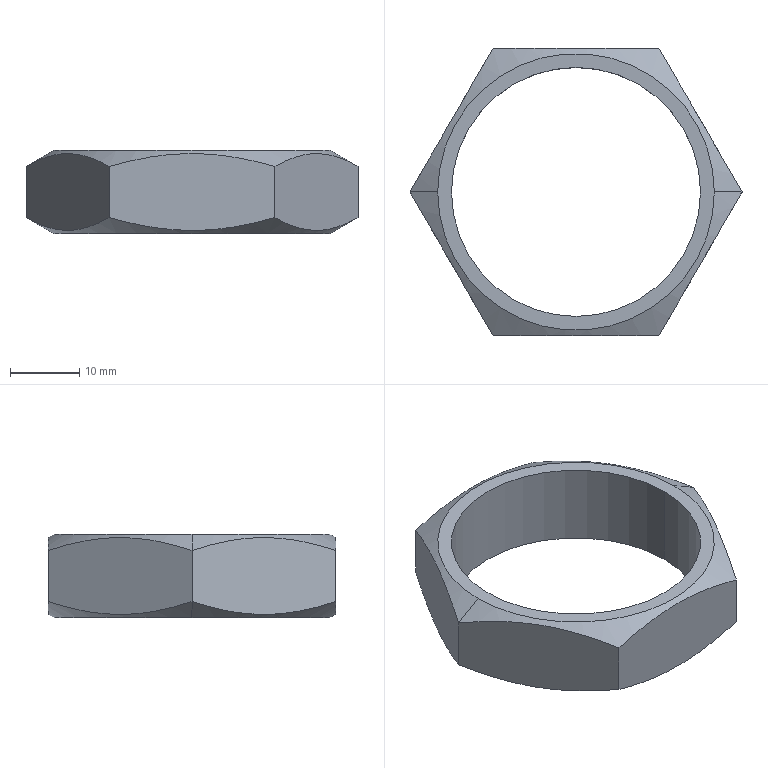Part | SolidWorks | features Extrusion 1, RevCut 1 | 1 solid | 14 faces | box 48 x 41.569 x 12 mm | volume 5415 mm3 | plane 8 | cone 4 | cylinder 2 | commonest cylinder face diameters 36 x2
STEP:
#1=CARTESIAN_POINT('',(-20.,0.,12.));
#2=VERTEX_POINT('',#1);
#3=CARTESIAN_POINT('',(20.,0.,12.));
#4=VERTEX_POINT('',#3);
#5=CARTESIAN_POINT('',(0.,0.,12.));
#6=DIRECTION('',(0.,0.,-1.));
#7=DIRECTION('',(-1.,0.,0.));
#8=AXIS2_PLACEMENT_3D('',#5,#6,#7);
#9=CIRCLE('',#8,20.);
#10=EDGE_CURVE('',#2,#4,#9,.T.);
#11=ORIENTED_EDGE('',*,*,#10,.T.);
#12=CARTESIAN_POINT('',(24.,0.,9.691));
#13=VERTEX_POINT('',#12);
#14=CARTESIAN_POINT('',(20.,0.,12.));
#15=DIRECTION('',(0.866,0.,-0.5));
#16=VECTOR('',#15,1000.);
#17=LINE('',#14,#16);
#18=EDGE_CURVE('',#4,#13,#17,.T.);
#19=ORIENTED_EDGE('',*,*,#18,.T.);
#20=CARTESIAN_POINT('',(12.,20.785,9.691));
#21=VERTEX_POINT('',#20);
#22=CARTESIAN_POINT('',(12.,20.785,9.691));
#23=CARTESIAN_POINT('',(12.98,19.088,10.256));
#24=CARTESIAN_POINT('',(13.967,17.379,10.722));
#25=CARTESIAN_POINT('',(15.961,13.924,11.368));
#26=CARTESIAN_POINT('',(16.968,12.179,11.546));
#27=CARTESIAN_POINT('',(18.244,9.97,11.547));
#28=CARTESIAN_POINT('',(18.5,9.526,11.537));
#29=CARTESIAN_POINT('',(19.01,8.642,11.494));
#30=CARTESIAN_POINT('',(19.265,8.202,11.462));
#31=CARTESIAN_POINT('',(20.025,6.885,11.335));
#32=CARTESIAN_POINT('',(20.528,6.013,11.209));
#33=CARTESIAN_POINT('',(22.03,3.412,10.724));
#34=CARTESIAN_POINT('',(23.019,1.699,10.257));
#35=CARTESIAN_POINT('',(24.,0.,9.691));
#36=B_SPLINE_CURVE_WITH_KNOTS('',3,(#22,#23,#24,#25,#26,#27,#28,#29,#30,#31,#32,#33,#34,#35),.UNSPECIFIED.,.F.,.F.,(4,2,2,2,2,2,4),(0.000000238,0.00606,0.01212,0.01363,0.01515,0.01818,0.02424),.UNSPECIFIED.);
#37=EDGE_CURVE('',#21,#13,#36,.T.);
#38=ORIENTED_EDGE('',*,*,#37,.F.);
#39=CARTESIAN_POINT('',(-12.,20.785,9.691));
#40=VERTEX_POINT('',#39);
#41=CARTESIAN_POINT('',(-12.,20.785,9.691));
#42=CARTESIAN_POINT('',(-11.024,20.785,9.972));
#43=CARTESIAN_POINT('',(-10.039,20.785,10.231));
#44=CARTESIAN_POINT('',(-8.046,20.785,10.69));
#45=CARTESIAN_POINT('',(-7.046,20.785,10.888));
#46=CARTESIAN_POINT('',(-4.04,20.785,11.373));
#47=CARTESIAN_POINT('',(-2.025,20.785,11.547));
#48=CARTESIAN_POINT('',(1.018,20.785,11.547));
#49=CARTESIAN_POINT('',(2.035,20.785,11.504));
#50=CARTESIAN_POINT('',(4.076,20.785,11.332));
#51=CARTESIAN_POINT('',(5.089,20.785,11.205));
#52=CARTESIAN_POINT('',(8.095,20.785,10.717));
#53=CARTESIAN_POINT('',(10.06,20.785,10.251));
#54=CARTESIAN_POINT('',(12.,20.785,9.691));
#55=B_SPLINE_CURVE_WITH_KNOTS('',3,(#41,#42,#43,#44,#45,#46,#47,#48,#49,#50,#51,#52,#53,#54),.UNSPECIFIED.,.F.,.F.,(4,2,2,2,2,2,4),(0.02134,0.02438,0.02741,0.03348,0.03652,0.03955,0.04562),.UNSPECIFIED.);
#56=EDGE_CURVE('',#40,#21,#55,.T.);
#57=ORIENTED_EDGE('',*,*,#56,.F.);
#58=CARTESIAN_POINT('',(-24.,0.,9.691));
#59=VERTEX_POINT('',#58);
#60=CARTESIAN_POINT('',(-24.,0.,9.691));
#61=CARTESIAN_POINT('',(-23.02,1.697,10.256));
#62=CARTESIAN_POINT('',(-22.033,3.406,10.722));
#63=CARTESIAN_POINT('',(-20.039,6.86,11.368));
#64=CARTESIAN_POINT('',(-19.032,8.605,11.546));
#65=CARTESIAN_POINT('',(-17.756,10.814,11.547));
#66=CARTESIAN_POINT('',(-17.5,11.258,11.537));
#67=CARTESIAN_POINT('',(-16.99,12.142,11.494));
#68=CARTESIAN_POINT('',(-16.735,12.583,11.462));
#69=CARTESIAN_POINT('',(-15.975,13.9,11.335));
#70=CARTESIAN_POINT('',(-15.472,14.772,11.209));
#71=CARTESIAN_POINT('',(-13.97,17.372,10.724));
#72=CARTESIAN_POINT('',(-12.981,19.086,10.257));
#73=CARTESIAN_POINT('',(-12.,20.785,9.691));
#74=B_SPLINE_CURVE_WITH_KNOTS('',3,(#60,#61,#62,#63,#64,#65,#66,#67,#68,#69,#70,#71,#72,#73),.UNSPECIFIED.,.F.,.F.,(4,2,2,2,2,2,4),(0.000000238,0.00606,0.01212,0.01363,0.01515,0.01818,0.02424),.UNSPECIFIED.);
#75=EDGE_CURVE('',#59,#40,#74,.T.);
#76=ORIENTED_EDGE('',*,*,#75,.F.);
#77=CARTESIAN_POINT('',(-20.,0.,12.));
#78=DIRECTION('',(-0.866,0.,-0.5));
#79=VECTOR('',#78,1000.);
#80=LINE('',#77,#79);
#81=EDGE_CURVE('',#2,#59,#80,.T.);
#82=ORIENTED_EDGE('',*,*,#81,.F.);
#83=EDGE_LOOP('',(#11,#19,#38,#57,#76,#82));
#84=FACE_OUTER_BOUND('',#83,.T.);
#85=CARTESIAN_POINT('',(0.,0.,12.));
#86=DIRECTION('',(0.,0.,-1.));
#87=DIRECTION('',(-1.,0.,0.));
#88=AXIS2_PLACEMENT_3D('',#85,#86,#87);
#89=CONICAL_SURFACE('',#88,20.,1.047);
#90=ADVANCED_FACE('',(#84),#89,.T.);
#91=CARTESIAN_POINT('',(-20.,0.,0.));
#92=VERTEX_POINT('',#91);
#93=CARTESIAN_POINT('',(20.,0.,0.));
#94=VERTEX_POINT('',#93);
#95=CARTESIAN_POINT('',(0.,0.,0.));
#96=DIRECTION('',(0.,0.,-1.));
#97=DIRECTION('',(-1.,0.,0.));
#98=AXIS2_PLACEMENT_3D('',#95,#96,#97);
#99=CIRCLE('',#98,20.);
#100=EDGE_CURVE('',#92,#94,#99,.T.);
#101=ORIENTED_EDGE('',*,*,#100,.F.);
#102=CARTESIAN_POINT('',(-24.,0.,2.309));
#103=VERTEX_POINT('',#102);
#104=CARTESIAN_POINT('',(-24.,0.,2.309));
#105=DIRECTION('',(-0.866,0.,0.5));
#106=VECTOR('',#105,1000.);
#107=LINE('',#104,#106);
#108=EDGE_CURVE('',#92,#103,#107,.T.);
#109=ORIENTED_EDGE('',*,*,#108,.T.);
#110=CARTESIAN_POINT('',(-12.,20.785,2.309));
#111=VERTEX_POINT('',#110);
#112=CARTESIAN_POINT('',(-12.,20.785,2.309));
#113=CARTESIAN_POINT('',(-12.98,19.088,1.744));
#114=CARTESIAN_POINT('',(-13.967,17.379,1.278));
#115=CARTESIAN_POINT('',(-15.961,13.924,0.6318));
#116=CARTESIAN_POINT('',(-16.968,12.179,0.4543));
#117=CARTESIAN_POINT('',(-18.244,9.97,0.4527));
#118=CARTESIAN_POINT('',(-18.5,9.526,0.4633));
#119=CARTESIAN_POINT('',(-19.01,8.642,0.506));
#120=CARTESIAN_POINT('',(-19.265,8.202,0.538));
#121=CARTESIAN_POINT('',(-20.025,6.885,0.6649));
#122=CARTESIAN_POINT('',(-20.528,6.013,0.7906));
#123=CARTESIAN_POINT('',(-22.03,3.412,1.276));
#124=CARTESIAN_POINT('',(-23.019,1.699,1.743));
#125=CARTESIAN_POINT('',(-24.,0.,2.309));
#126=B_SPLINE_CURVE_WITH_KNOTS('',3,(#112,#113,#114,#115,#116,#117,#118,#119,#120,#121,#122,#123,#124,#125),.UNSPECIFIED.,.F.,.F.,(4,2,2,2,2,2,4),(0.000000238,0.00606,0.01212,0.01363,0.01515,0.01818,0.02424),.UNSPECIFIED.);
#127=EDGE_CURVE('',#111,#103,#126,.T.);
#128=ORIENTED_EDGE('',*,*,#127,.F.);
#129=CARTESIAN_POINT('',(12.,20.785,2.309));
#130=VERTEX_POINT('',#129);
#131=CARTESIAN_POINT('',(12.,20.785,2.309));
#132=CARTESIAN_POINT('',(10.06,20.785,1.749));
#133=CARTESIAN_POINT('',(8.095,20.785,1.283));
#134=CARTESIAN_POINT('',(5.089,20.785,0.795));
#135=CARTESIAN_POINT('',(4.076,20.785,0.6676));
#136=CARTESIAN_POINT('',(2.035,20.785,0.4963));
#137=CARTESIAN_POINT('',(1.018,20.785,0.4531));
#138=CARTESIAN_POINT('',(-2.025,20.785,0.4528));
#139=CARTESIAN_POINT('',(-4.04,20.785,0.627));
#140=CARTESIAN_POINT('',(-7.046,20.785,1.112));
#141=CARTESIAN_POINT('',(-8.046,20.785,1.31));
#142=CARTESIAN_POINT('',(-10.039,20.785,1.769));
#143=CARTESIAN_POINT('',(-11.024,20.785,2.028));
#144=CARTESIAN_POINT('',(-12.,20.785,2.309));
#145=B_SPLINE_CURVE_WITH_KNOTS('',3,(#131,#132,#133,#134,#135,#136,#137,#138,#139,#140,#141,#142,#143,#144),.UNSPECIFIED.,.F.,.F.,(4,2,2,2,2,2,4),(0.008871,0.01493,0.01796,0.02098,0.02704,0.03007,0.0331),.UNSPECIFIED.);
#146=EDGE_CURVE('',#130,#111,#145,.T.);
#147=ORIENTED_EDGE('',*,*,#146,.F.);
#148=CARTESIAN_POINT('',(24.,0.,2.309));
#149=VERTEX_POINT('',#148);
#150=CARTESIAN_POINT('',(24.,0.,2.309));
#151=CARTESIAN_POINT('',(23.02,1.697,1.744));
#152=CARTESIAN_POINT('',(22.033,3.406,1.278));
#153=CARTESIAN_POINT('',(20.039,6.86,0.6318));
#154=CARTESIAN_POINT('',(19.032,8.605,0.4543));
#155=CARTESIAN_POINT('',(17.756,10.814,0.4527));
#156=CARTESIAN_POINT('',(17.5,11.258,0.4633));
#157=CARTESIAN_POINT('',(16.99,12.142,0.506));
#158=CARTESIAN_POINT('',(16.735,12.583,0.538));
#159=CARTESIAN_POINT('',(15.975,13.9,0.6649));
#160=CARTESIAN_POINT('',(15.472,14.772,0.7906));
#161=CARTESIAN_POINT('',(13.97,17.372,1.276));
#162=CARTESIAN_POINT('',(12.981,19.086,1.743));
#163=CARTESIAN_POINT('',(12.,20.785,2.309));
#164=B_SPLINE_CURVE_WITH_KNOTS('',3,(#150,#151,#152,#153,#154,#155,#156,#157,#158,#159,#160,#161,#162,#163),.UNSPECIFIED.,.F.,.F.,(4,2,2,2,2,2,4),(0.000000238,0.00606,0.01212,0.01363,0.01515,0.01818,0.02424),.UNSPECIFIED.);
#165=EDGE_CURVE('',#149,#130,#164,.T.);
#166=ORIENTED_EDGE('',*,*,#165,.F.);
#167=CARTESIAN_POINT('',(24.,0.,2.309));
#168=DIRECTION('',(0.866,0.,0.5));
#169=VECTOR('',#168,1000.);
#170=LINE('',#167,#169);
#171=EDGE_CURVE('',#94,#149,#170,.T.);
#172=ORIENTED_EDGE('',*,*,#171,.F.);
#173=EDGE_LOOP('',(#101,#109,#128,#147,#166,#172));
#174=FACE_OUTER_BOUND('',#173,.T.);
#175=CARTESIAN_POINT('',(0.,0.,2.309));
#176=DIRECTION('',(0.,0.,1.));
#177=DIRECTION('',(1.,0.,0.));
#178=AXIS2_PLACEMENT_3D('',#175,#176,#177);
#179=CONICAL_SURFACE('',#178,24.,1.047);
#180=ADVANCED_FACE('',(#174),#179,.T.);
#181=CARTESIAN_POINT('',(-18.,0.,12.));
#182=VERTEX_POINT('',#181);
#183=CARTESIAN_POINT('',(18.,0.,12.));
#184=VERTEX_POINT('',#183);
#185=CARTESIAN_POINT('',(0.,0.,12.));
#186=DIRECTION('',(0.,0.,1.));
#187=DIRECTION('',(1.,0.,0.));
#188=AXIS2_PLACEMENT_3D('',#185,#186,#187);
#189=CIRCLE('',#188,18.);
#190=EDGE_CURVE('',#182,#184,#189,.T.);
#191=ORIENTED_EDGE('',*,*,#190,.T.);
#192=CARTESIAN_POINT('',(18.,0.,0.));
#193=VERTEX_POINT('',#192);
#194=CARTESIAN_POINT('',(18.,0.,12.));
#195=DIRECTION('',(0.,0.,-1.));
#196=VECTOR('',#195,1000.);
#197=LINE('',#194,#196);
#198=EDGE_CURVE('',#184,#193,#197,.T.);
#199=ORIENTED_EDGE('',*,*,#198,.T.);
#200=CARTESIAN_POINT('',(-18.,0.,0.));
#201=VERTEX_POINT('',#200);
#202=CARTESIAN_POINT('',(0.,0.,0.));
#203=DIRECTION('',(0.,0.,1.));
#204=DIRECTION('',(1.,0.,0.));
#205=AXIS2_PLACEMENT_3D('',#202,#203,#204);
#206=CIRCLE('',#205,18.);
#207=EDGE_CURVE('',#201,#193,#206,.T.);
#208=ORIENTED_EDGE('',*,*,#207,.F.);
#209=CARTESIAN_POINT('',(-18.,0.,12.));
#210=DIRECTION('',(0.,0.,-1.));
#211=VECTOR('',#210,1000.);
#212=LINE('',#209,#211);
#213=EDGE_CURVE('',#182,#201,#212,.T.);
#214=ORIENTED_EDGE('',*,*,#213,.F.);
#215=EDGE_LOOP('',(#191,#199,#208,#214));
#216=FACE_OUTER_BOUND('',#215,.T.);
#217=CARTESIAN_POINT('',(0.,0.,12.));
#218=DIRECTION('',(0.,0.,-1.));
#219=DIRECTION('',(-1.,0.,0.));
#220=AXIS2_PLACEMENT_3D('',#217,#218,#219);
#221=CYLINDRICAL_SURFACE('',#220,18.);
#222=ADVANCED_FACE('',(#216),#221,.F.);
#223=ORIENTED_EDGE('',*,*,#207,.T.);
#224=CARTESIAN_POINT('',(0.,0.,0.));
#225=DIRECTION('',(0.,0.,1.));
#226=DIRECTION('',(1.,0.,0.));
#227=AXIS2_PLACEMENT_3D('',#224,#225,#226);
#228=CIRCLE('',#227,18.);
#229=EDGE_CURVE('',#193,#201,#228,.T.);
#230=ORIENTED_EDGE('',*,*,#229,.T.);
#231=EDGE_LOOP('',(#223,#230));
#232=FACE_BOUND('',#231,.T.);
#233=CARTESIAN_POINT('',(0.,0.,0.));
#234=DIRECTION('',(0.,0.,-1.));
#235=DIRECTION('',(-1.,0.,0.));
#236=AXIS2_PLACEMENT_3D('',#233,#234,#235);
#237=CIRCLE('',#236,20.);
#238=EDGE_CURVE('',#94,#92,#237,.T.);
#239=ORIENTED_EDGE('',*,*,#238,.T.);
#240=ORIENTED_EDGE('',*,*,#100,.T.);
#241=EDGE_LOOP('',(#239,#240));
#242=FACE_OUTER_BOUND('',#241,.T.);
#243=CARTESIAN_POINT('',(0.,0.,0.));
#244=DIRECTION('',(0.,0.,1.));
#245=DIRECTION('',(1.,0.,0.));
#246=AXIS2_PLACEMENT_3D('',#243,#244,#245);
#247=PLANE('',#246);
#248=ADVANCED_FACE('',(#232,#242),#247,.F.);
#249=ORIENTED_EDGE('',*,*,#10,.F.);
#250=CARTESIAN_POINT('',(0.,0.,12.));
#251=DIRECTION('',(0.,0.,-1.));
#252=DIRECTION('',(-1.,0.,0.));
#253=AXIS2_PLACEMENT_3D('',#250,#251,#252);
#254=CIRCLE('',#253,20.);
#255=EDGE_CURVE('',#4,#2,#254,.T.);
#256=ORIENTED_EDGE('',*,*,#255,.F.);
#257=EDGE_LOOP('',(#249,#256));
#258=FACE_OUTER_BOUND('',#257,.T.);
#259=ORIENTED_EDGE('',*,*,#190,.F.);
#260=CARTESIAN_POINT('',(0.,0.,12.));
#261=DIRECTION('',(0.,0.,1.));
#262=DIRECTION('',(1.,0.,0.));
#263=AXIS2_PLACEMENT_3D('',#260,#261,#262);
#264=CIRCLE('',#263,18.);
#265=EDGE_CURVE('',#184,#182,#264,.T.);
#266=ORIENTED_EDGE('',*,*,#265,.F.);
#267=EDGE_LOOP('',(#259,#266));
#268=FACE_BOUND('',#267,.T.);
#269=CARTESIAN_POINT('',(0.,0.,12.));
#270=DIRECTION('',(0.,0.,1.));
#271=DIRECTION('',(1.,0.,0.));
#272=AXIS2_PLACEMENT_3D('',#269,#270,#271);
#273=PLANE('',#272);
#274=ADVANCED_FACE('',(#258,#268),#273,.T.);
#275=CARTESIAN_POINT('',(24.,0.,12.));
#276=DIRECTION('',(0.,0.,-1.));
#277=VECTOR('',#276,1000.);
#278=LINE('',#275,#277);
#279=EDGE_CURVE('',#13,#149,#278,.T.);
#280=ORIENTED_EDGE('',*,*,#279,.F.);
#281=CARTESIAN_POINT('',(12.,-20.785,9.691));
#282=VERTEX_POINT('',#281);
#283=CARTESIAN_POINT('',(24.,0.,9.691));
#284=CARTESIAN_POINT('',(23.02,-1.697,10.256));
#285=CARTESIAN_POINT('',(22.033,-3.406,10.722));
#286=CARTESIAN_POINT('',(20.039,-6.86,11.368));
#287=CARTESIAN_POINT('',(19.032,-8.605,11.546));
#288=CARTESIAN_POINT('',(17.756,-10.814,11.547));
#289=CARTESIAN_POINT('',(17.5,-11.258,11.537));
#290=CARTESIAN_POINT('',(16.99,-12.142,11.494));
#291=CARTESIAN_POINT('',(16.735,-12.583,11.462));
#292=CARTESIAN_POINT('',(15.975,-13.9,11.335));
#293=CARTESIAN_POINT('',(15.472,-14.772,11.209));
#294=CARTESIAN_POINT('',(13.97,-17.372,10.724));
#295=CARTESIAN_POINT('',(12.981,-19.086,10.257));
#296=CARTESIAN_POINT('',(12.,-20.785,9.691));
#297=B_SPLINE_CURVE_WITH_KNOTS('',3,(#283,#284,#285,#286,#287,#288,#289,#290,#291,#292,#293,#294,#295,#296),.UNSPECIFIED.,.F.,.F.,(4,2,2,2,2,2,4),(0.000000238,0.00606,0.01212,0.01363,0.01515,0.01818,0.02424),.UNSPECIFIED.);
#298=EDGE_CURVE('',#13,#282,#297,.T.);
#299=ORIENTED_EDGE('',*,*,#298,.T.);
#300=CARTESIAN_POINT('',(12.,-20.785,2.309));
#301=VERTEX_POINT('',#300);
#302=CARTESIAN_POINT('',(12.,-20.785,12.));
#303=DIRECTION('',(0.,0.,-1.));
#304=VECTOR('',#303,1000.);
#305=LINE('',#302,#304);
#306=EDGE_CURVE('',#282,#301,#305,.T.);
#307=ORIENTED_EDGE('',*,*,#306,.T.);
#308=CARTESIAN_POINT('',(12.,-20.785,2.309));
#309=CARTESIAN_POINT('',(12.98,-19.088,1.744));
#310=CARTESIAN_POINT('',(13.967,-17.379,1.278));
#311=CARTESIAN_POINT('',(15.961,-13.924,0.6318));
#312=CARTESIAN_POINT('',(16.968,-12.179,0.4543));
#313=CARTESIAN_POINT('',(18.244,-9.97,0.4527));
#314=CARTESIAN_POINT('',(18.5,-9.526,0.4633));
#315=CARTESIAN_POINT('',(19.01,-8.642,0.506));
#316=CARTESIAN_POINT('',(19.265,-8.202,0.538));
#317=CARTESIAN_POINT('',(20.025,-6.885,0.6649));
#318=CARTESIAN_POINT('',(20.528,-6.013,0.7906));
#319=CARTESIAN_POINT('',(22.03,-3.412,1.276));
#320=CARTESIAN_POINT('',(23.019,-1.699,1.743));
#321=CARTESIAN_POINT('',(24.,0.,2.309));
#322=B_SPLINE_CURVE_WITH_KNOTS('',3,(#308,#309,#310,#311,#312,#313,#314,#315,#316,#317,#318,#319,#320,#321),.UNSPECIFIED.,.F.,.F.,(4,2,2,2,2,2,4),(0.000000238,0.00606,0.01212,0.01363,0.01515,0.01818,0.02424),.UNSPECIFIED.);
#323=EDGE_CURVE('',#301,#149,#322,.T.);
#324=ORIENTED_EDGE('',*,*,#323,.T.);
#325=EDGE_LOOP('',(#280,#299,#307,#324));
#326=FACE_OUTER_BOUND('',#325,.T.);
#327=CARTESIAN_POINT('',(12.,-20.785,12.));
#328=DIRECTION('',(-0.866,0.5,0.));
#329=DIRECTION('',(-0.5,-0.866,0.));
#330=AXIS2_PLACEMENT_3D('',#327,#328,#329);
#331=PLANE('',#330);
#332=ADVANCED_FACE('',(#326),#331,.F.);
#333=CARTESIAN_POINT('',(12.,20.785,12.));
#334=DIRECTION('',(0.,0.,-1.));
#335=VECTOR('',#334,1000.);
#336=LINE('',#333,#335);
#337=EDGE_CURVE('',#21,#130,#336,.T.);
#338=ORIENTED_EDGE('',*,*,#337,.F.);
#339=ORIENTED_EDGE('',*,*,#37,.T.);
#340=ORIENTED_EDGE('',*,*,#279,.T.);
#341=ORIENTED_EDGE('',*,*,#165,.T.);
#342=EDGE_LOOP('',(#338,#339,#340,#341));
#343=FACE_OUTER_BOUND('',#342,.T.);
#344=CARTESIAN_POINT('',(24.,0.,12.));
#345=DIRECTION('',(-0.866,-0.5,0.));
#346=DIRECTION('',(0.5,-0.866,0.));
#347=AXIS2_PLACEMENT_3D('',#344,#345,#346);
#348=PLANE('',#347);
#349=ADVANCED_FACE('',(#343),#348,.F.);
#350=CARTESIAN_POINT('',(-12.,20.785,12.));
#351=DIRECTION('',(0.,0.,-1.));
#352=VECTOR('',#351,1000.);
#353=LINE('',#350,#352);
#354=EDGE_CURVE('',#40,#111,#353,.T.);
#355=ORIENTED_EDGE('',*,*,#354,.F.);
#356=ORIENTED_EDGE('',*,*,#56,.T.);
#357=ORIENTED_EDGE('',*,*,#337,.T.);
#358=ORIENTED_EDGE('',*,*,#146,.T.);
#359=EDGE_LOOP('',(#355,#356,#357,#358));
#360=FACE_OUTER_BOUND('',#359,.T.);
#361=CARTESIAN_POINT('',(12.,20.785,12.));
#362=DIRECTION('',(0.,-1.,0.));
#363=DIRECTION('',(0.,0.,-1.));
#364=AXIS2_PLACEMENT_3D('',#361,#362,#363);
#365=PLANE('',#364);
#366=ADVANCED_FACE('',(#360),#365,.F.);
#367=CARTESIAN_POINT('',(-24.,0.,12.));
#368=DIRECTION('',(0.,0.,-1.));
#369=VECTOR('',#368,1000.);
#370=LINE('',#367,#369);
#371=EDGE_CURVE('',#59,#103,#370,.T.);
#372=ORIENTED_EDGE('',*,*,#371,.F.);
#373=ORIENTED_EDGE('',*,*,#75,.T.);
#374=ORIENTED_EDGE('',*,*,#354,.T.);
#375=ORIENTED_EDGE('',*,*,#127,.T.);
#376=EDGE_LOOP('',(#372,#373,#374,#375));
#377=FACE_OUTER_BOUND('',#376,.T.);
#378=CARTESIAN_POINT('',(-12.,20.785,12.));
#379=DIRECTION('',(0.866,-0.5,0.));
#380=DIRECTION('',(0.5,0.866,0.));
#381=AXIS2_PLACEMENT_3D('',#378,#379,#380);
#382=PLANE('',#381);
#383=ADVANCED_FACE('',(#377),#382,.F.);
#384=CARTESIAN_POINT('',(-12.,-20.785,9.691));
#385=VERTEX_POINT('',#384);
#386=CARTESIAN_POINT('',(-12.,-20.785,2.309));
#387=VERTEX_POINT('',#386);
#388=CARTESIAN_POINT('',(-12.,-20.785,12.));
#389=DIRECTION('',(0.,0.,-1.));
#390=VECTOR('',#389,1000.);
#391=LINE('',#388,#390);
#392=EDGE_CURVE('',#385,#387,#391,.T.);
#393=ORIENTED_EDGE('',*,*,#392,.F.);
#394=CARTESIAN_POINT('',(-12.,-20.785,9.691));
#395=CARTESIAN_POINT('',(-12.98,-19.088,10.256));
#396=CARTESIAN_POINT('',(-13.967,-17.379,10.722));
#397=CARTESIAN_POINT('',(-15.961,-13.924,11.368));
#398=CARTESIAN_POINT('',(-16.968,-12.179,11.546));
#399=CARTESIAN_POINT('',(-18.244,-9.97,11.547));
#400=CARTESIAN_POINT('',(-18.5,-9.526,11.537));
#401=CARTESIAN_POINT('',(-19.01,-8.642,11.494));
#402=CARTESIAN_POINT('',(-19.265,-8.202,11.462));
#403=CARTESIAN_POINT('',(-20.025,-6.885,11.335));
#404=CARTESIAN_POINT('',(-20.528,-6.013,11.209));
#405=CARTESIAN_POINT('',(-22.03,-3.412,10.724));
#406=CARTESIAN_POINT('',(-23.019,-1.699,10.257));
#407=CARTESIAN_POINT('',(-24.,0.,9.691));
#408=B_SPLINE_CURVE_WITH_KNOTS('',3,(#394,#395,#396,#397,#398,#399,#400,#401,#402,#403,#404,#405,#406,#407),.UNSPECIFIED.,.F.,.F.,(4,2,2,2,2,2,4),(0.000000238,0.00606,0.01212,0.01363,0.01515,0.01818,0.02424),.UNSPECIFIED.);
#409=EDGE_CURVE('',#385,#59,#408,.T.);
#410=ORIENTED_EDGE('',*,*,#409,.T.);
#411=ORIENTED_EDGE('',*,*,#371,.T.);
#412=CARTESIAN_POINT('',(-24.,0.,2.309));
#413=CARTESIAN_POINT('',(-23.02,-1.697,1.744));
#414=CARTESIAN_POINT('',(-22.033,-3.406,1.278));
#415=CARTESIAN_POINT('',(-20.039,-6.86,0.6318));
#416=CARTESIAN_POINT('',(-19.032,-8.605,0.4543));
#417=CARTESIAN_POINT('',(-17.756,-10.814,0.4527));
#418=CARTESIAN_POINT('',(-17.5,-11.258,0.4633));
#419=CARTESIAN_POINT('',(-16.99,-12.142,0.506));
#420=CARTESIAN_POINT('',(-16.735,-12.583,0.538));
#421=CARTESIAN_POINT('',(-15.975,-13.9,0.6649));
#422=CARTESIAN_POINT('',(-15.472,-14.772,0.7906));
#423=CARTESIAN_POINT('',(-13.97,-17.372,1.276));
#424=CARTESIAN_POINT('',(-12.981,-19.086,1.743));
#425=CARTESIAN_POINT('',(-12.,-20.785,2.309));
#426=B_SPLINE_CURVE_WITH_KNOTS('',3,(#412,#413,#414,#415,#416,#417,#418,#419,#420,#421,#422,#423,#424,#425),.UNSPECIFIED.,.F.,.F.,(4,2,2,2,2,2,4),(0.000000238,0.00606,0.01212,0.01363,0.01515,0.01818,0.02424),.UNSPECIFIED.);
#427=EDGE_CURVE('',#103,#387,#426,.T.);
#428=ORIENTED_EDGE('',*,*,#427,.T.);
#429=EDGE_LOOP('',(#393,#410,#411,#428));
#430=FACE_OUTER_BOUND('',#429,.T.);
#431=CARTESIAN_POINT('',(-24.,0.,12.));
#432=DIRECTION('',(0.866,0.5,0.));
#433=DIRECTION('',(-0.5,0.866,0.));
#434=AXIS2_PLACEMENT_3D('',#431,#432,#433);
#435=PLANE('',#434);
#436=ADVANCED_FACE('',(#430),#435,.F.);
#437=ORIENTED_EDGE('',*,*,#306,.F.);
#438=CARTESIAN_POINT('',(12.,-20.785,9.691));
#439=CARTESIAN_POINT('',(10.06,-20.785,10.251));
#440=CARTESIAN_POINT('',(8.095,-20.785,10.717));
#441=CARTESIAN_POINT('',(5.089,-20.785,11.205));
#442=CARTESIAN_POINT('',(4.076,-20.785,11.332));
#443=CARTESIAN_POINT('',(2.035,-20.785,11.504));
#444=CARTESIAN_POINT('',(1.018,-20.785,11.547));
#445=CARTESIAN_POINT('',(-2.025,-20.785,11.547));
#446=CARTESIAN_POINT('',(-4.04,-20.785,11.373));
#447=CARTESIAN_POINT('',(-7.046,-20.785,10.888));
#448=CARTESIAN_POINT('',(-8.046,-20.785,10.69));
#449=CARTESIAN_POINT('',(-10.039,-20.785,10.231));
#450=CARTESIAN_POINT('',(-11.024,-20.785,9.972));
#451=CARTESIAN_POINT('',(-12.,-20.785,9.691));
#452=B_SPLINE_CURVE_WITH_KNOTS('',3,(#438,#439,#440,#441,#442,#443,#444,#445,#446,#447,#448,#449,#450,#451),.UNSPECIFIED.,.F.,.F.,(4,2,2,2,2,2,4),(0.008871,0.01493,0.01796,0.02098,0.02704,0.03007,0.0331),.UNSPECIFIED.);
#453=EDGE_CURVE('',#282,#385,#452,.T.);
#454=ORIENTED_EDGE('',*,*,#453,.T.);
#455=ORIENTED_EDGE('',*,*,#392,.T.);
#456=CARTESIAN_POINT('',(-12.,-20.785,2.309));
#457=CARTESIAN_POINT('',(-11.024,-20.785,2.028));
#458=CARTESIAN_POINT('',(-10.039,-20.785,1.769));
#459=CARTESIAN_POINT('',(-8.046,-20.785,1.31));
#460=CARTESIAN_POINT('',(-7.046,-20.785,1.112));
#461=CARTESIAN_POINT('',(-4.04,-20.785,0.627));
#462=CARTESIAN_POINT('',(-2.025,-20.785,0.4528));
#463=CARTESIAN_POINT('',(1.018,-20.785,0.4531));
#464=CARTESIAN_POINT('',(2.035,-20.785,0.4963));
#465=CARTESIAN_POINT('',(4.076,-20.785,0.6676));
#466=CARTESIAN_POINT('',(5.089,-20.785,0.795));
#467=CARTESIAN_POINT('',(8.095,-20.785,1.283));
#468=CARTESIAN_POINT('',(10.06,-20.785,1.749));
#469=CARTESIAN_POINT('',(12.,-20.785,2.309));
#470=B_SPLINE_CURVE_WITH_KNOTS('',3,(#456,#457,#458,#459,#460,#461,#462,#463,#464,#465,#466,#467,#468,#469),.UNSPECIFIED.,.F.,.F.,(4,2,2,2,2,2,4),(0.02134,0.02438,0.02741,0.03348,0.03652,0.03955,0.04562),.UNSPECIFIED.);
#471=EDGE_CURVE('',#387,#301,#470,.T.);
#472=ORIENTED_EDGE('',*,*,#471,.T.);
#473=EDGE_LOOP('',(#437,#454,#455,#472));
#474=FACE_OUTER_BOUND('',#473,.T.);
#475=CARTESIAN_POINT('',(-12.,-20.785,12.));
#476=DIRECTION('',(0.,1.,0.));
#477=DIRECTION('',(0.,0.,1.));
#478=AXIS2_PLACEMENT_3D('',#475,#476,#477);
#479=PLANE('',#478);
#480=ADVANCED_FACE('',(#474),#479,.F.);
#481=ORIENTED_EDGE('',*,*,#198,.F.);
#482=ORIENTED_EDGE('',*,*,#265,.T.);
#483=ORIENTED_EDGE('',*,*,#213,.T.);
#484=ORIENTED_EDGE('',*,*,#229,.F.);
#485=EDGE_LOOP('',(#481,#482,#483,#484));
#486=FACE_OUTER_BOUND('',#485,.T.);
#487=CARTESIAN_POINT('',(0.,0.,12.));
#488=DIRECTION('',(0.,0.,-1.));
#489=DIRECTION('',(-1.,0.,0.));
#490=AXIS2_PLACEMENT_3D('',#487,#488,#489);
#491=CYLINDRICAL_SURFACE('',#490,18.);
#492=ADVANCED_FACE('',(#486),#491,.F.);
#493=ORIENTED_EDGE('',*,*,#108,.F.);
#494=ORIENTED_EDGE('',*,*,#238,.F.);
#495=ORIENTED_EDGE('',*,*,#171,.T.);
#496=ORIENTED_EDGE('',*,*,#323,.F.);
#497=ORIENTED_EDGE('',*,*,#471,.F.);
#498=ORIENTED_EDGE('',*,*,#427,.F.);
#499=EDGE_LOOP('',(#493,#494,#495,#496,#497,#498));
#500=FACE_OUTER_BOUND('',#499,.T.);
#501=CARTESIAN_POINT('',(0.,0.,2.309));
#502=DIRECTION('',(0.,0.,1.));
#503=DIRECTION('',(1.,0.,0.));
#504=AXIS2_PLACEMENT_3D('',#501,#502,#503);
#505=CONICAL_SURFACE('',#504,24.,1.047);
#506=ADVANCED_FACE('',(#500),#505,.T.);
#507=ORIENTED_EDGE('',*,*,#18,.F.);
#508=ORIENTED_EDGE('',*,*,#255,.T.);
#509=ORIENTED_EDGE('',*,*,#81,.T.);
#510=ORIENTED_EDGE('',*,*,#409,.F.);
#511=ORIENTED_EDGE('',*,*,#453,.F.);
#512=ORIENTED_EDGE('',*,*,#298,.F.);
#513=EDGE_LOOP('',(#507,#508,#509,#510,#511,#512));
#514=FACE_OUTER_BOUND('',#513,.T.);
#515=CARTESIAN_POINT('',(0.,0.,12.));
#516=DIRECTION('',(0.,0.,-1.));
#517=DIRECTION('',(-1.,0.,0.));
#518=AXIS2_PLACEMENT_3D('',#515,#516,#517);
#519=CONICAL_SURFACE('',#518,20.,1.047);
#520=ADVANCED_FACE('',(#514),#519,.T.);
#521=CLOSED_SHELL('',(#90,#180,#222,#248,#274,#332,#349,#366,#383,#436,#480,#492,#506,#520));
#522=MANIFOLD_SOLID_BREP('',#521);
#523=CARTESIAN_POINT('',(0.,0.,0.));
#524=DIRECTION('',(0.,0.,1.));
#525=DIRECTION('',(1.,0.,0.));
#526=AXIS2_PLACEMENT_3D('',#523,#524,#525);
#527=(LENGTH_UNIT()NAMED_UNIT(*)SI_UNIT(.MILLI.,.METRE.));
#528=UNCERTAINTY_MEASURE_WITH_UNIT(LENGTH_MEASURE(0.00001),#527,'','');
#529=(NAMED_UNIT(*)PLANE_ANGLE_UNIT()SI_UNIT($,.RADIAN.));
#530=(NAMED_UNIT(*)SI_UNIT($,.STERADIAN.)SOLID_ANGLE_UNIT());
#531=(GEOMETRIC_REPRESENTATION_CONTEXT(3)GLOBAL_UNCERTAINTY_ASSIGNED_CONTEXT((#528))GLOBAL_UNIT_ASSIGNED_CONTEXT((#527,#529,#530))REPRESENTATION_CONTEXT('',''));
#532=ADVANCED_BREP_SHAPE_REPRESENTATION('',(#522,#526),#531);